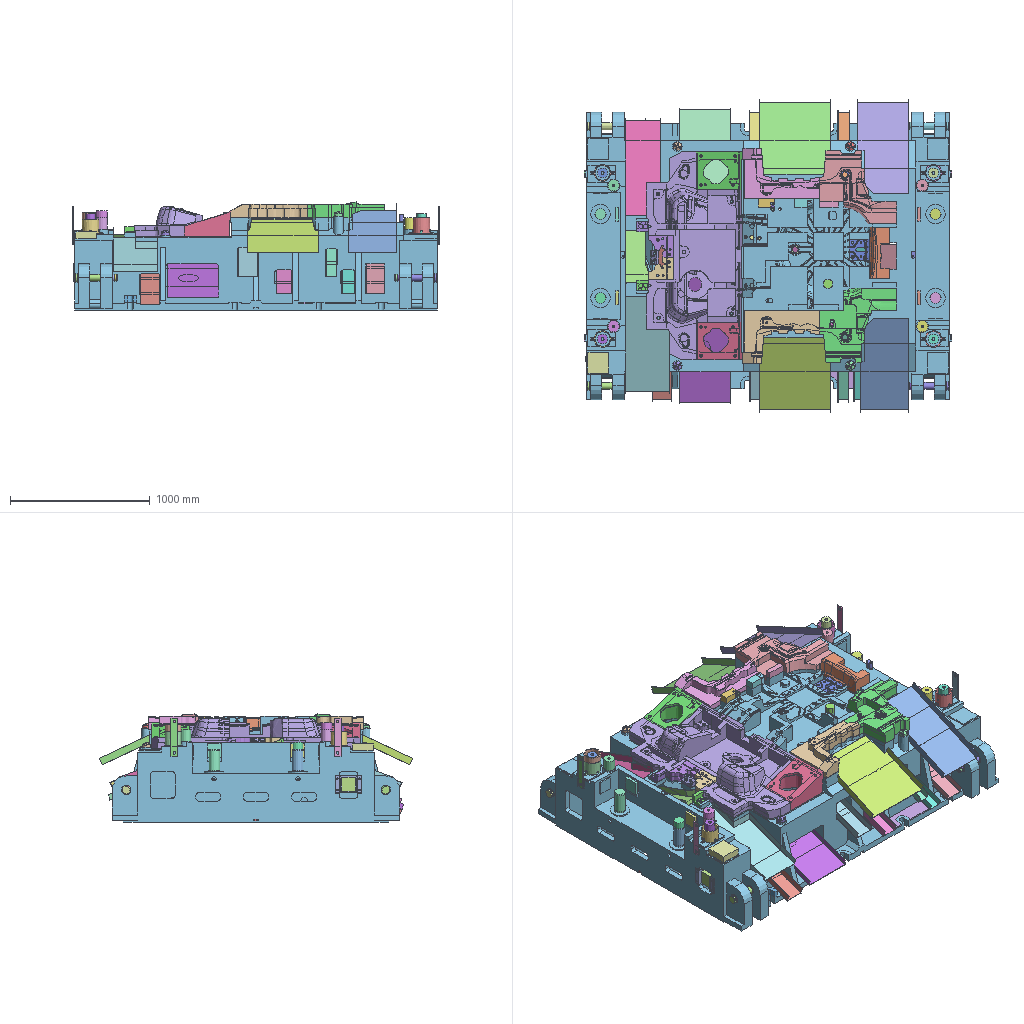Assembly | NX | 111 different items | 111 placed | box 2630 x 2247 x 774 mm
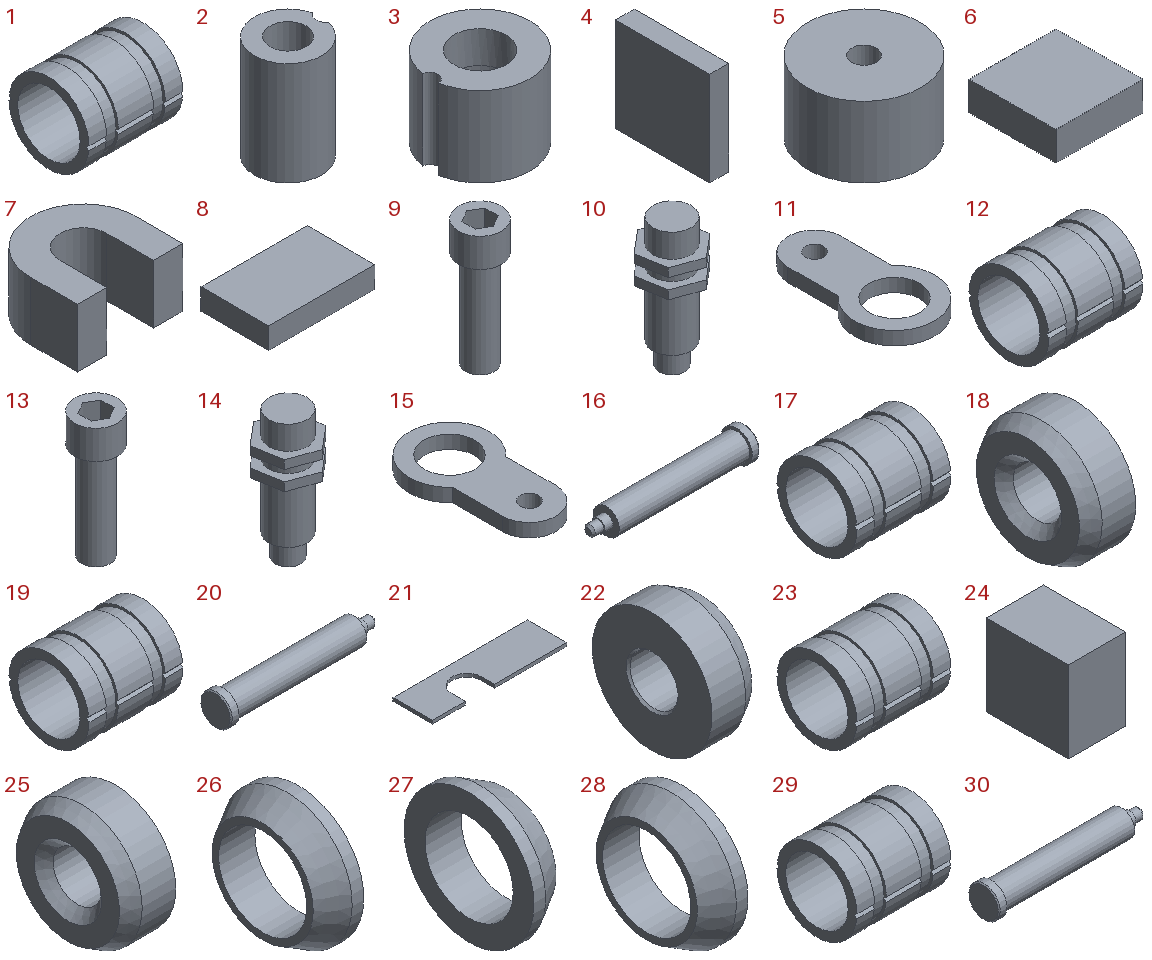Parts list (item | quantity | size | volume | features):
1 | x1 | 80 x 67.999 x 68 mm | 105275 mm3 | features solid 2
2 | x1 | 12.8 x 13 x 20 mm | 1637 mm3 | features solid 2
3 | x1 | 24.84 x 25 x 20 mm | 6037 mm3 | features solid 2
4 | x1 | 20 x 100 x 100 mm | 200000 mm3 | features solid 2
5 | x1 | 80 x 80 x 50 mm | 239301 mm3 | features solid 2
6 | x1 | 150 x 150 x 50 mm | 1125000 mm3 | features solid 2
7 | x1 | 90 x 85 x 50 mm | 227627 mm3 | features solid 2
8 | x1 | 50 x 32 x 10 mm | 16000 mm3 | features solid 2
9 | x1 | 9 x 9 x 26 mm | 875.359 mm3 | features solid 2
10 | x1 | 26.042 x 27.292 x 60 mm | 15809 mm3 | features solid 2
11 | x1 | 30 x 55 x 5 mm | 4330 mm3 | features solid 2
12 | x1 | 80 x 67.999 x 68 mm | 105275 mm3 | features solid 2
13 | x1 | 9 x 9 x 26 mm | 875.359 mm3 | features solid 2
14 | x1 | 26.042 x 27.292 x 60 mm | 15809 mm3 | features solid 2
15 | x1 | 30 x 55 x 5 mm | 4330 mm3 | features solid 2
16 | x1 | 300 x 60 x 60 mm | 546127 mm3 | features solid 2
17 | x1 | 80 x 67.999 x 68 mm | 105275 mm3 | features solid 2
18 | x1 | 20 x 50 x 50 mm | 30708 mm3 | features solid 2
19 | x1 | 80 x 67.999 x 68 mm | 105275 mm3 | features solid 2
20 | x1 | 300 x 60 x 60 mm | 546127 mm3 | features solid 2
21 | x1 | 410 x 120 x 10 mm | 424191 mm3 | features solid 2
22 | x1 | 20 x 50 x 50 mm | 30708 mm3 | features solid 2
23 | x1 | 80 x 67.999 x 68 mm | 105275 mm3 | features solid 2
24 | x1 | 70 x 100 x 100 mm | 700000 mm3 | features solid 2
25 | x1 | 20 x 50 x 50 mm | 30708 mm3 | features solid 2
26 | x1 | 14 x 50 x 50 mm | 10965 mm3 | features solid 2
27 | x1 | 14 x 50 x 50 mm | 10965 mm3 | features solid 2
28 | x1 | 14 x 50 x 50 mm | 10965 mm3 | features solid 2
29 | x1 | 80 x 67.999 x 68 mm | 105275 mm3 | features solid 2
30 | x1 | 300 x 60 x 60 mm | 546127 mm3 | features solid 2
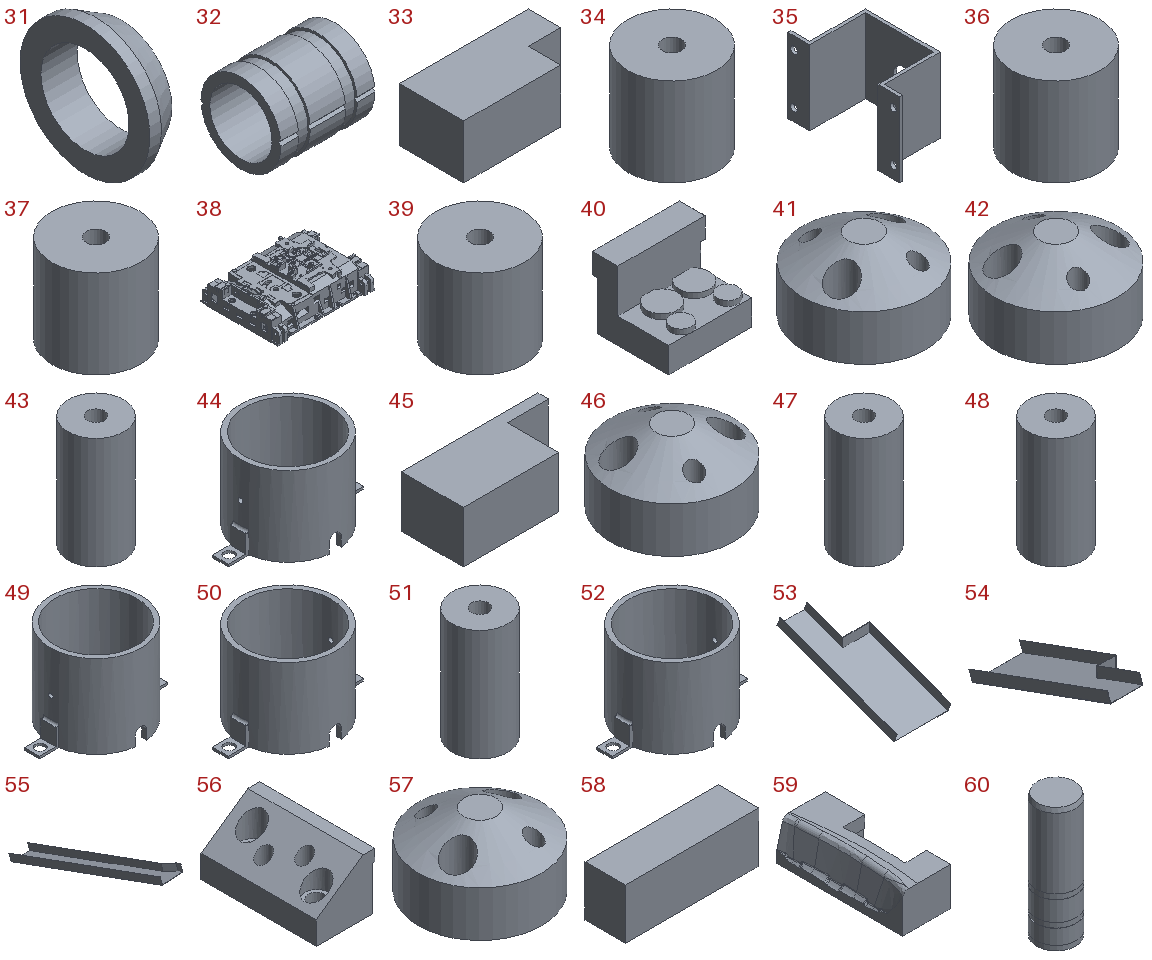31 | x1 | 14 x 50 x 50 mm | 10965 mm3 | features solid 2
32 | x1 | 80 x 67.999 x 68 mm | 105275 mm3 | features solid 2
33 | x1 | 120 x 60 x 50 mm | 314985 mm3 | features solid 2
34 | x1 | 80 x 80 x 80 mm | 385615 mm3 | features solid 2
35 | x1 | 95 x 180 x 120 mm | 210565 mm3 | features solid 2
36 | x1 | 80 x 80 x 80 mm | 385615 mm3 | features solid 2
37 | x1 | 80 x 80 x 80 mm | 385615 mm3 | features solid 2
38 | x1 | 2620 x 2060 x 758 mm | 857197509 mm3 | features solid 2
39 | x1 | 80 x 80 x 80 mm | 385615 mm3 | features solid 2
40 | x1 | 85.559 x 74.968 x 67.5 mm | 231490 mm3 | features solid 2
41 | x1 | 60 x 60 x 35 mm | 69581 mm3 | features solid 2
42 | x1 | 60 x 60 x 35 mm | 69581 mm3 | features solid 2
43 | x1 | 70 x 70 x 140 mm | 490293 mm3 | features solid 2
44 | x1 | 170 x 120 x 100 mm | 216597 mm3 | features solid 2
45 | x1 | 132.49 x 60 x 50 mm | 297471 mm3 | features solid 2
46 | x1 | 60 x 60 x 35 mm | 69581 mm3 | features solid 2
47 | x1 | 70 x 70 x 140 mm | 490293 mm3 | features solid 2
48 | x1 | 70 x 70 x 140 mm | 490293 mm3 | features solid 2
49 | x1 | 170 x 120 x 110 mm | 238085 mm3 | features solid 2
50 | x1 | 170 x 120 x 100 mm | 216597 mm3 | features solid 2
51 | x1 | 70 x 70 x 140 mm | 490293 mm3 | features solid 2
52 | x1 | 170 x 120 x 100 mm | 216597 mm3 | features solid 2
53 | x1 | 315 x 695.354 x 293.848 mm | 535547 mm3 | features solid 2
54 | x1 | 250 x 695.354 x 293.848 mm | 465781 mm3 | features solid 2
55 | x1 | 175.737 x 1183 x 471.211 mm | 600196 mm3 | features solid 2
56 | x1 | 50 x 98.314 x 47.5 mm | 148836 mm3 | features solid 2
57 | x1 | 60 x 60 x 35 mm | 69581 mm3 | features solid 2
58 | x1 | 132.5 x 40 x 50 mm | 265000 mm3 | features solid 2
59 | x1 | 140.004 x 365 x 111 mm | 4062417 mm3 | features solid 2
60 | x1 | 80 x 80 x 250 mm | 1250401 mm3 | features solid 2
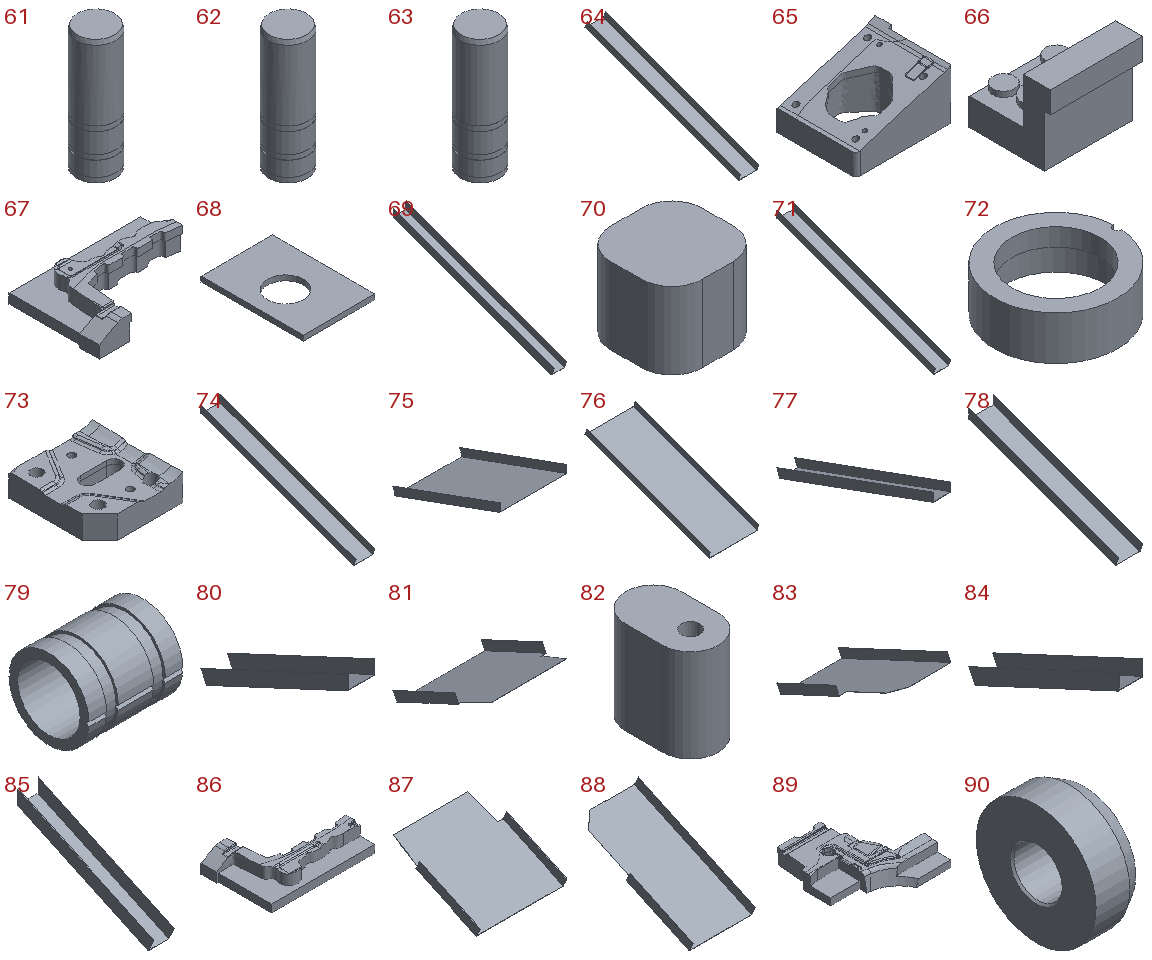61 | x1 | 80 x 80 x 250 mm | 1250401 mm3 | features solid 2
62 | x1 | 80 x 80 x 250 mm | 1250401 mm3 | features solid 2
63 | x1 | 80 x 80 x 250 mm | 1250401 mm3 | features solid 2
64 | x1 | 133.224 x 1128 x 451.241 mm | 541870 mm3 | features solid 2
65 | x1 | 335 x 270 x 179.884 mm | 7620802 mm3 | features solid 2
66 | x1 | 85.559 x 74.968 x 67.5 mm | 231490 mm3 | features solid 2
67 | x1 | 550.001 x 380 x 97 mm | 6391201 mm3 | features solid 2
68 | x1 | 140 x 200 x 10 mm | 241515 mm3 | features solid 2
69 | x1 | 90 x 1127 x 457.216 mm | 441303 mm3 | features solid 2
70 | x1 | 60 x 60 x 50 mm | 162831 mm3 | features solid 2
71 | x1 | 110 x 1127 x 457.216 mm | 488567 mm3 | features solid 2
72 | x1 | 55.929 x 56 x 20 mm | 19140 mm3 | features solid 2
73 | x1 | 142.5 x 155.001 x 45.841 mm | 709213 mm3 | features solid 2
74 | x1 | 140 x 1127 x 457.216 mm | 559463 mm3 | features solid 2
75 | x1 | 365 x 582.65 x 252.914 mm | 321613 mm3 | features solid 2
76 | x1 | 365 x 936.307 x 376.531 mm | 517909 mm3 | features solid 2
77 | x1 | 110 x 957.101 x 395.341 mm | 414032 mm3 | features solid 2
78 | x1 | 140 x 857.101 x 358.944 mm | 423844 mm3 | features solid 2
79 | x1 | 80 x 67.999 x 68 mm | 105275 mm3 | features solid 2
80 | x1 | 105 x 571.131 x 311.638 mm | 246383 mm3 | features solid 2
81 | x1 | 510 x 538.761 x 242.084 mm | 358465 mm3 | features solid 2
82 | x1 | 30 x 50 x 50 mm | 61416 mm3 | features solid 2
83 | x1 | 370 x 674.707 x 350.792 mm | 358626 mm3 | features solid 2
84 | x1 | 85 x 521.131 x 288.323 mm | 202118 mm3 | features solid 2
85 | x1 | 80 x 521.131 x 288.323 mm | 196597 mm3 | features solid 2
86 | x1 | 550 x 360 x 97 mm | 5944260 mm3 | features solid 2
87 | x1 | 510 x 538.761 x 242.084 mm | 358465 mm3 | features solid 2
88 | x1 | 350 x 674.707 x 350.792 mm | 350900 mm3 | features solid 2
89 | x1 | 552.249 x 525 x 114.078 mm | 11768272 mm3 | features solid 2
90 | x1 | 20 x 50 x 50 mm | 30708 mm3 | features solid 2
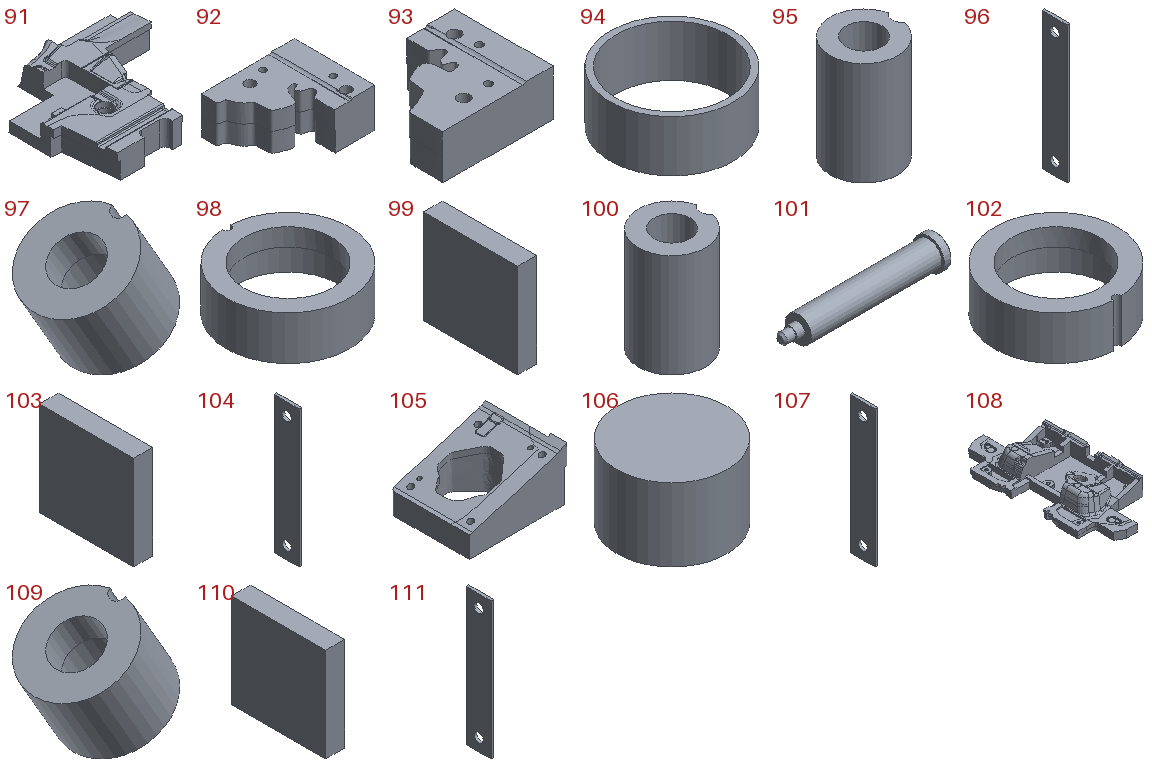91 | x1 | 552.249 x 535.003 x 114.074 mm | 12312889 mm3 | features solid 2
92 | x1 | 179.483 x 155 x 75 mm | 1313323 mm3 | features solid 2
93 | x1 | 179.985 x 160 x 75 mm | 1451097 mm3 | features solid 2
94 | x1 | 120 x 120 x 50 mm | 107442 mm3 | features solid 2
95 | x1 | 12.8 x 13 x 20 mm | 1637 mm3 | features solid 2
96 | x1 | 5 x 50 x 275 mm | 66205 mm3 | features solid 2
97 | x1 | 31.555 x 25 x 29.766 mm | 6194 mm3 | features solid 2
98 | x1 | 56 x 55.929 x 20 mm | 19140 mm3 | features solid 2
99 | x1 | 20 x 100 x 100 mm | 200000 mm3 | features solid 2
100 | x1 | 12.8 x 13 x 20 mm | 1637 mm3 | features solid 2
101 | x1 | 300 x 60 x 60 mm | 546127 mm3 | features solid 2
102 | x1 | 56 x 55.929 x 20 mm | 19140 mm3 | features solid 2
103 | x1 | 20 x 100 x 100 mm | 200000 mm3 | features solid 2
104 | x1 | 5 x 50 x 275 mm | 66205 mm3 | features solid 2
105 | x1 | 335 x 270 x 179.884 mm | 7603778 mm3 | features solid 2
106 | x1 | 75.347 x 75.347 x 50 mm | 222939 mm3 | features solid 2
107 | x1 | 5 x 50 x 275 mm | 66205 mm3 | features solid 2
108 | x1 | 690.824 x 1490 x 210.501 mm | 61253517 mm3 | features solid 2
109 | x1 | 31.532 x 25 x 29.752 mm | 6194 mm3 | features solid 2
110 | x1 | 20 x 100 x 100 mm | 200000 mm3 | features solid 2
111 | x1 | 5 x 50 x 275 mm | 66205 mm3 | features solid 2